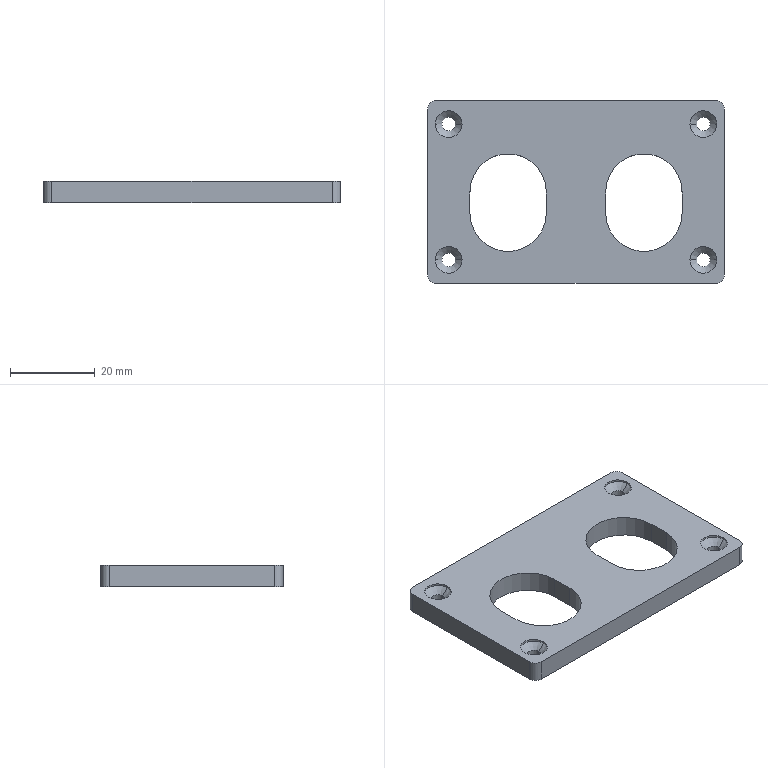Part | SolidWorks | features Extrusion 1, HoleWzd 1 | 1 solid | 42 faces | box 70 x 43 x 5 mm | volume 11317 mm3 | cylinder 24 | plane 10 | cone 8 | commonest cylinder face diameters 3.2 x8 6.3 x8 4 x4 18 x4
STEP:
#1=CARTESIAN_POINT('',(1.85,37.5,4.5));
#2=VERTEX_POINT('',#1);
#3=CARTESIAN_POINT('',(8.15,37.5,4.5));
#4=VERTEX_POINT('',#3);
#5=CARTESIAN_POINT('',(5.,37.5,4.5));
#6=DIRECTION('',(0.,0.,1.));
#7=DIRECTION('',(1.,0.,0.));
#8=AXIS2_PLACEMENT_3D('',#5,#6,#7);
#9=CIRCLE('',#8,3.15);
#10=EDGE_CURVE('',#2,#4,#9,.T.);
#11=ORIENTED_EDGE('',*,*,#10,.F.);
#12=CARTESIAN_POINT('',(1.85,37.5,5.));
#13=VERTEX_POINT('',#12);
#14=CARTESIAN_POINT('',(1.85,37.5,5.));
#15=DIRECTION('',(0.,0.,1.));
#16=VECTOR('',#15,1000.);
#17=LINE('',#14,#16);
#18=EDGE_CURVE('',#2,#13,#17,.T.);
#19=ORIENTED_EDGE('',*,*,#18,.T.);
#20=CARTESIAN_POINT('',(8.15,37.5,5.));
#21=VERTEX_POINT('',#20);
#22=CARTESIAN_POINT('',(5.,37.5,5.));
#23=DIRECTION('',(0.,0.,1.));
#24=DIRECTION('',(1.,0.,0.));
#25=AXIS2_PLACEMENT_3D('',#22,#23,#24);
#26=CIRCLE('',#25,3.15);
#27=EDGE_CURVE('',#13,#21,#26,.T.);
#28=ORIENTED_EDGE('',*,*,#27,.T.);
#29=CARTESIAN_POINT('',(8.15,37.5,5.));
#30=DIRECTION('',(0.,0.,1.));
#31=VECTOR('',#30,1000.);
#32=LINE('',#29,#31);
#33=EDGE_CURVE('',#4,#21,#32,.T.);
#34=ORIENTED_EDGE('',*,*,#33,.F.);
#35=EDGE_LOOP('',(#11,#19,#28,#34));
#36=FACE_OUTER_BOUND('',#35,.T.);
#37=CARTESIAN_POINT('',(5.,37.5,5.));
#38=DIRECTION('',(0.,0.,1.));
#39=DIRECTION('',(1.,0.,0.));
#40=AXIS2_PLACEMENT_3D('',#37,#38,#39);
#41=CYLINDRICAL_SURFACE('',#40,3.15);
#42=ADVANCED_FACE('',(#36),#41,.F.);
#43=CARTESIAN_POINT('',(3.4,37.5,2.95));
#44=VERTEX_POINT('',#43);
#45=CARTESIAN_POINT('',(6.6,37.5,2.95));
#46=VERTEX_POINT('',#45);
#47=CARTESIAN_POINT('',(5.,37.5,2.95));
#48=DIRECTION('',(0.,0.,1.));
#49=DIRECTION('',(1.,0.,0.));
#50=AXIS2_PLACEMENT_3D('',#47,#48,#49);
#51=CIRCLE('',#50,1.6);
#52=EDGE_CURVE('',#44,#46,#51,.T.);
#53=ORIENTED_EDGE('',*,*,#52,.F.);
#54=CARTESIAN_POINT('',(1.85,37.5,4.5));
#55=DIRECTION('',(-0.7071,0.,0.7071));
#56=VECTOR('',#55,1000.);
#57=LINE('',#54,#56);
#58=EDGE_CURVE('',#44,#2,#57,.T.);
#59=ORIENTED_EDGE('',*,*,#58,.T.);
#60=ORIENTED_EDGE('',*,*,#10,.T.);
#61=CARTESIAN_POINT('',(8.15,37.5,4.5));
#62=DIRECTION('',(0.7071,0.,0.7071));
#63=VECTOR('',#62,1000.);
#64=LINE('',#61,#63);
#65=EDGE_CURVE('',#46,#4,#64,.T.);
#66=ORIENTED_EDGE('',*,*,#65,.F.);
#67=EDGE_LOOP('',(#53,#59,#60,#66));
#68=FACE_OUTER_BOUND('',#67,.T.);
#69=CARTESIAN_POINT('',(5.,37.5,4.5));
#70=DIRECTION('',(0.,0.,1.));
#71=DIRECTION('',(1.,0.,0.));
#72=AXIS2_PLACEMENT_3D('',#69,#70,#71);
#73=CONICAL_SURFACE('',#72,3.15,0.7854);
#74=ADVANCED_FACE('',(#68),#73,.F.);
#75=CARTESIAN_POINT('',(3.4,37.5,0.));
#76=VERTEX_POINT('',#75);
#77=CARTESIAN_POINT('',(6.6,37.5,0.));
#78=VERTEX_POINT('',#77);
#79=CARTESIAN_POINT('',(5.,37.5,0.));
#80=DIRECTION('',(0.,0.,1.));
#81=DIRECTION('',(1.,0.,0.));
#82=AXIS2_PLACEMENT_3D('',#79,#80,#81);
#83=CIRCLE('',#82,1.6);
#84=EDGE_CURVE('',#76,#78,#83,.T.);
#85=ORIENTED_EDGE('',*,*,#84,.F.);
#86=CARTESIAN_POINT('',(3.4,37.5,5.));
#87=DIRECTION('',(0.,0.,1.));
#88=VECTOR('',#87,1000.);
#89=LINE('',#86,#88);
#90=EDGE_CURVE('',#76,#44,#89,.T.);
#91=ORIENTED_EDGE('',*,*,#90,.T.);
#92=ORIENTED_EDGE('',*,*,#52,.T.);
#93=CARTESIAN_POINT('',(6.6,37.5,5.));
#94=DIRECTION('',(0.,0.,1.));
#95=VECTOR('',#94,1000.);
#96=LINE('',#93,#95);
#97=EDGE_CURVE('',#78,#46,#96,.T.);
#98=ORIENTED_EDGE('',*,*,#97,.F.);
#99=EDGE_LOOP('',(#85,#91,#92,#98));
#100=FACE_OUTER_BOUND('',#99,.T.);
#101=CARTESIAN_POINT('',(5.,37.5,5.));
#102=DIRECTION('',(0.,0.,1.));
#103=DIRECTION('',(1.,0.,0.));
#104=AXIS2_PLACEMENT_3D('',#101,#102,#103);
#105=CYLINDRICAL_SURFACE('',#104,1.6);
#106=ADVANCED_FACE('',(#100),#105,.F.);
#107=CARTESIAN_POINT('',(1.85,5.5,4.5));
#108=VERTEX_POINT('',#107);
#109=CARTESIAN_POINT('',(8.15,5.5,4.5));
#110=VERTEX_POINT('',#109);
#111=CARTESIAN_POINT('',(5.,5.5,4.5));
#112=DIRECTION('',(0.,0.,1.));
#113=DIRECTION('',(1.,0.,0.));
#114=AXIS2_PLACEMENT_3D('',#111,#112,#113);
#115=CIRCLE('',#114,3.15);
#116=EDGE_CURVE('',#108,#110,#115,.T.);
#117=ORIENTED_EDGE('',*,*,#116,.F.);
#118=CARTESIAN_POINT('',(1.85,5.5,5.));
#119=VERTEX_POINT('',#118);
#120=CARTESIAN_POINT('',(1.85,5.5,5.));
#121=DIRECTION('',(0.,0.,1.));
#122=VECTOR('',#121,1000.);
#123=LINE('',#120,#122);
#124=EDGE_CURVE('',#108,#119,#123,.T.);
#125=ORIENTED_EDGE('',*,*,#124,.T.);
#126=CARTESIAN_POINT('',(8.15,5.5,5.));
#127=VERTEX_POINT('',#126);
#128=CARTESIAN_POINT('',(5.,5.5,5.));
#129=DIRECTION('',(0.,0.,1.));
#130=DIRECTION('',(1.,0.,0.));
#131=AXIS2_PLACEMENT_3D('',#128,#129,#130);
#132=CIRCLE('',#131,3.15);
#133=EDGE_CURVE('',#119,#127,#132,.T.);
#134=ORIENTED_EDGE('',*,*,#133,.T.);
#135=CARTESIAN_POINT('',(8.15,5.5,5.));
#136=DIRECTION('',(0.,0.,1.));
#137=VECTOR('',#136,1000.);
#138=LINE('',#135,#137);
#139=EDGE_CURVE('',#110,#127,#138,.T.);
#140=ORIENTED_EDGE('',*,*,#139,.F.);
#141=EDGE_LOOP('',(#117,#125,#134,#140));
#142=FACE_OUTER_BOUND('',#141,.T.);
#143=CARTESIAN_POINT('',(5.,5.5,5.));
#144=DIRECTION('',(0.,0.,1.));
#145=DIRECTION('',(1.,0.,0.));
#146=AXIS2_PLACEMENT_3D('',#143,#144,#145);
#147=CYLINDRICAL_SURFACE('',#146,3.15);
#148=ADVANCED_FACE('',(#142),#147,.F.);
#149=CARTESIAN_POINT('',(3.4,5.5,2.95));
#150=VERTEX_POINT('',#149);
#151=CARTESIAN_POINT('',(6.6,5.5,2.95));
#152=VERTEX_POINT('',#151);
#153=CARTESIAN_POINT('',(5.,5.5,2.95));
#154=DIRECTION('',(0.,0.,1.));
#155=DIRECTION('',(1.,0.,0.));
#156=AXIS2_PLACEMENT_3D('',#153,#154,#155);
#157=CIRCLE('',#156,1.6);
#158=EDGE_CURVE('',#150,#152,#157,.T.);
#159=ORIENTED_EDGE('',*,*,#158,.F.);
#160=CARTESIAN_POINT('',(1.85,5.5,4.5));
#161=DIRECTION('',(-0.7071,0.,0.7071));
#162=VECTOR('',#161,1000.);
#163=LINE('',#160,#162);
#164=EDGE_CURVE('',#150,#108,#163,.T.);
#165=ORIENTED_EDGE('',*,*,#164,.T.);
#166=ORIENTED_EDGE('',*,*,#116,.T.);
#167=CARTESIAN_POINT('',(8.15,5.5,4.5));
#168=DIRECTION('',(0.7071,0.,0.7071));
#169=VECTOR('',#168,1000.);
#170=LINE('',#167,#169);
#171=EDGE_CURVE('',#152,#110,#170,.T.);
#172=ORIENTED_EDGE('',*,*,#171,.F.);
#173=EDGE_LOOP('',(#159,#165,#166,#172));
#174=FACE_OUTER_BOUND('',#173,.T.);
#175=CARTESIAN_POINT('',(5.,5.5,4.5));
#176=DIRECTION('',(0.,0.,1.));
#177=DIRECTION('',(1.,0.,0.));
#178=AXIS2_PLACEMENT_3D('',#175,#176,#177);
#179=CONICAL_SURFACE('',#178,3.15,0.7854);
#180=ADVANCED_FACE('',(#174),#179,.F.);
#181=CARTESIAN_POINT('',(3.4,5.5,0.));
#182=VERTEX_POINT('',#181);
#183=CARTESIAN_POINT('',(6.6,5.5,0.));
#184=VERTEX_POINT('',#183);
#185=CARTESIAN_POINT('',(5.,5.5,0.));
#186=DIRECTION('',(0.,0.,1.));
#187=DIRECTION('',(1.,0.,0.));
#188=AXIS2_PLACEMENT_3D('',#185,#186,#187);
#189=CIRCLE('',#188,1.6);
#190=EDGE_CURVE('',#182,#184,#189,.T.);
#191=ORIENTED_EDGE('',*,*,#190,.F.);
#192=CARTESIAN_POINT('',(3.4,5.5,5.));
#193=DIRECTION('',(0.,0.,1.));
#194=VECTOR('',#193,1000.);
#195=LINE('',#192,#194);
#196=EDGE_CURVE('',#182,#150,#195,.T.);
#197=ORIENTED_EDGE('',*,*,#196,.T.);
#198=ORIENTED_EDGE('',*,*,#158,.T.);
#199=CARTESIAN_POINT('',(6.6,5.5,5.));
#200=DIRECTION('',(0.,0.,1.));
#201=VECTOR('',#200,1000.);
#202=LINE('',#199,#201);
#203=EDGE_CURVE('',#184,#152,#202,.T.);
#204=ORIENTED_EDGE('',*,*,#203,.F.);
#205=EDGE_LOOP('',(#191,#197,#198,#204));
#206=FACE_OUTER_BOUND('',#205,.T.);
#207=CARTESIAN_POINT('',(5.,5.5,5.));
#208=DIRECTION('',(0.,0.,1.));
#209=DIRECTION('',(1.,0.,0.));
#210=AXIS2_PLACEMENT_3D('',#207,#208,#209);
#211=CYLINDRICAL_SURFACE('',#210,1.6);
#212=ADVANCED_FACE('',(#206),#211,.F.);
#213=CARTESIAN_POINT('',(61.85,5.5,4.5));
#214=VERTEX_POINT('',#213);
#215=CARTESIAN_POINT('',(68.15,5.5,4.5));
#216=VERTEX_POINT('',#215);
#217=CARTESIAN_POINT('',(65.,5.5,4.5));
#218=DIRECTION('',(0.,0.,1.));
#219=DIRECTION('',(1.,0.,0.));
#220=AXIS2_PLACEMENT_3D('',#217,#218,#219);
#221=CIRCLE('',#220,3.15);
#222=EDGE_CURVE('',#214,#216,#221,.T.);
#223=ORIENTED_EDGE('',*,*,#222,.F.);
#224=CARTESIAN_POINT('',(61.85,5.5,5.));
#225=VERTEX_POINT('',#224);
#226=CARTESIAN_POINT('',(61.85,5.5,5.));
#227=DIRECTION('',(0.,0.,1.));
#228=VECTOR('',#227,1000.);
#229=LINE('',#226,#228);
#230=EDGE_CURVE('',#214,#225,#229,.T.);
#231=ORIENTED_EDGE('',*,*,#230,.T.);
#232=CARTESIAN_POINT('',(68.15,5.5,5.));
#233=VERTEX_POINT('',#232);
#234=CARTESIAN_POINT('',(65.,5.5,5.));
#235=DIRECTION('',(0.,0.,1.));
#236=DIRECTION('',(1.,0.,0.));
#237=AXIS2_PLACEMENT_3D('',#234,#235,#236);
#238=CIRCLE('',#237,3.15);
#239=EDGE_CURVE('',#225,#233,#238,.T.);
#240=ORIENTED_EDGE('',*,*,#239,.T.);
#241=CARTESIAN_POINT('',(68.15,5.5,5.));
#242=DIRECTION('',(0.,0.,1.));
#243=VECTOR('',#242,1000.);
#244=LINE('',#241,#243);
#245=EDGE_CURVE('',#216,#233,#244,.T.);
#246=ORIENTED_EDGE('',*,*,#245,.F.);
#247=EDGE_LOOP('',(#223,#231,#240,#246));
#248=FACE_OUTER_BOUND('',#247,.T.);
#249=CARTESIAN_POINT('',(65.,5.5,5.));
#250=DIRECTION('',(0.,0.,1.));
#251=DIRECTION('',(1.,0.,0.));
#252=AXIS2_PLACEMENT_3D('',#249,#250,#251);
#253=CYLINDRICAL_SURFACE('',#252,3.15);
#254=ADVANCED_FACE('',(#248),#253,.F.);
#255=CARTESIAN_POINT('',(63.4,5.5,2.95));
#256=VERTEX_POINT('',#255);
#257=CARTESIAN_POINT('',(66.6,5.5,2.95));
#258=VERTEX_POINT('',#257);
#259=CARTESIAN_POINT('',(65.,5.5,2.95));
#260=DIRECTION('',(0.,0.,1.));
#261=DIRECTION('',(1.,0.,0.));
#262=AXIS2_PLACEMENT_3D('',#259,#260,#261);
#263=CIRCLE('',#262,1.6);
#264=EDGE_CURVE('',#256,#258,#263,.T.);
#265=ORIENTED_EDGE('',*,*,#264,.F.);
#266=CARTESIAN_POINT('',(61.85,5.5,4.5));
#267=DIRECTION('',(-0.7071,0.,0.7071));
#268=VECTOR('',#267,1000.);
#269=LINE('',#266,#268);
#270=EDGE_CURVE('',#256,#214,#269,.T.);
#271=ORIENTED_EDGE('',*,*,#270,.T.);
#272=ORIENTED_EDGE('',*,*,#222,.T.);
#273=CARTESIAN_POINT('',(68.15,5.5,4.5));
#274=DIRECTION('',(0.7071,0.,0.7071));
#275=VECTOR('',#274,1000.);
#276=LINE('',#273,#275);
#277=EDGE_CURVE('',#258,#216,#276,.T.);
#278=ORIENTED_EDGE('',*,*,#277,.F.);
#279=EDGE_LOOP('',(#265,#271,#272,#278));
#280=FACE_OUTER_BOUND('',#279,.T.);
#281=CARTESIAN_POINT('',(65.,5.5,4.5));
#282=DIRECTION('',(0.,0.,1.));
#283=DIRECTION('',(1.,0.,0.));
#284=AXIS2_PLACEMENT_3D('',#281,#282,#283);
#285=CONICAL_SURFACE('',#284,3.15,0.7854);
#286=ADVANCED_FACE('',(#280),#285,.F.);
#287=CARTESIAN_POINT('',(63.4,5.5,0.));
#288=VERTEX_POINT('',#287);
#289=CARTESIAN_POINT('',(66.6,5.5,0.));
#290=VERTEX_POINT('',#289);
#291=CARTESIAN_POINT('',(65.,5.5,0.));
#292=DIRECTION('',(0.,0.,1.));
#293=DIRECTION('',(1.,0.,0.));
#294=AXIS2_PLACEMENT_3D('',#291,#292,#293);
#295=CIRCLE('',#294,1.6);
#296=EDGE_CURVE('',#288,#290,#295,.T.);
#297=ORIENTED_EDGE('',*,*,#296,.F.);
#298=CARTESIAN_POINT('',(63.4,5.5,5.));
#299=DIRECTION('',(0.,0.,1.));
#300=VECTOR('',#299,1000.);
#301=LINE('',#298,#300);
#302=EDGE_CURVE('',#288,#256,#301,.T.);
#303=ORIENTED_EDGE('',*,*,#302,.T.);
#304=ORIENTED_EDGE('',*,*,#264,.T.);
#305=CARTESIAN_POINT('',(66.6,5.5,5.));
#306=DIRECTION('',(0.,0.,1.));
#307=VECTOR('',#306,1000.);
#308=LINE('',#305,#307);
#309=EDGE_CURVE('',#290,#258,#308,.T.);
#310=ORIENTED_EDGE('',*,*,#309,.F.);
#311=EDGE_LOOP('',(#297,#303,#304,#310));
#312=FACE_OUTER_BOUND('',#311,.T.);
#313=CARTESIAN_POINT('',(65.,5.5,5.));
#314=DIRECTION('',(0.,0.,1.));
#315=DIRECTION('',(1.,0.,0.));
#316=AXIS2_PLACEMENT_3D('',#313,#314,#315);
#317=CYLINDRICAL_SURFACE('',#316,1.6);
#318=ADVANCED_FACE('',(#312),#317,.F.);
#319=CARTESIAN_POINT('',(61.85,37.5,4.5));
#320=VERTEX_POINT('',#319);
#321=CARTESIAN_POINT('',(68.15,37.5,4.5));
#322=VERTEX_POINT('',#321);
#323=CARTESIAN_POINT('',(65.,37.5,4.5));
#324=DIRECTION('',(0.,0.,1.));
#325=DIRECTION('',(1.,0.,0.));
#326=AXIS2_PLACEMENT_3D('',#323,#324,#325);
#327=CIRCLE('',#326,3.15);
#328=EDGE_CURVE('',#320,#322,#327,.T.);
#329=ORIENTED_EDGE('',*,*,#328,.F.);
#330=CARTESIAN_POINT('',(61.85,37.5,5.));
#331=VERTEX_POINT('',#330);
#332=CARTESIAN_POINT('',(61.85,37.5,5.));
#333=DIRECTION('',(0.,0.,1.));
#334=VECTOR('',#333,1000.);
#335=LINE('',#332,#334);
#336=EDGE_CURVE('',#320,#331,#335,.T.);
#337=ORIENTED_EDGE('',*,*,#336,.T.);
#338=CARTESIAN_POINT('',(68.15,37.5,5.));
#339=VERTEX_POINT('',#338);
#340=CARTESIAN_POINT('',(65.,37.5,5.));
#341=DIRECTION('',(0.,0.,1.));
#342=DIRECTION('',(1.,0.,0.));
#343=AXIS2_PLACEMENT_3D('',#340,#341,#342);
#344=CIRCLE('',#343,3.15);
#345=EDGE_CURVE('',#331,#339,#344,.T.);
#346=ORIENTED_EDGE('',*,*,#345,.T.);
#347=CARTESIAN_POINT('',(68.15,37.5,5.));
#348=DIRECTION('',(0.,0.,1.));
#349=VECTOR('',#348,1000.);
#350=LINE('',#347,#349);
#351=EDGE_CURVE('',#322,#339,#350,.T.);
#352=ORIENTED_EDGE('',*,*,#351,.F.);
#353=EDGE_LOOP('',(#329,#337,#346,#352));
#354=FACE_OUTER_BOUND('',#353,.T.);
#355=CARTESIAN_POINT('',(65.,37.5,5.));
#356=DIRECTION('',(0.,0.,1.));
#357=DIRECTION('',(1.,0.,0.));
#358=AXIS2_PLACEMENT_3D('',#355,#356,#357);
#359=CYLINDRICAL_SURFACE('',#358,3.15);
#360=ADVANCED_FACE('',(#354),#359,.F.);
#361=CARTESIAN_POINT('',(63.4,37.5,2.95));
#362=VERTEX_POINT('',#361);
#363=CARTESIAN_POINT('',(66.6,37.5,2.95));
#364=VERTEX_POINT('',#363);
#365=CARTESIAN_POINT('',(65.,37.5,2.95));
#366=DIRECTION('',(0.,0.,1.));
#367=DIRECTION('',(1.,0.,0.));
#368=AXIS2_PLACEMENT_3D('',#365,#366,#367);
#369=CIRCLE('',#368,1.6);
#370=EDGE_CURVE('',#362,#364,#369,.T.);
#371=ORIENTED_EDGE('',*,*,#370,.F.);
#372=CARTESIAN_POINT('',(61.85,37.5,4.5));
#373=DIRECTION('',(-0.7071,0.,0.7071));
#374=VECTOR('',#373,1000.);
#375=LINE('',#372,#374);
#376=EDGE_CURVE('',#362,#320,#375,.T.);
#377=ORIENTED_EDGE('',*,*,#376,.T.);
#378=ORIENTED_EDGE('',*,*,#328,.T.);
#379=CARTESIAN_POINT('',(68.15,37.5,4.5));
#380=DIRECTION('',(0.7071,0.,0.7071));
#381=VECTOR('',#380,1000.);
#382=LINE('',#379,#381);
#383=EDGE_CURVE('',#364,#322,#382,.T.);
#384=ORIENTED_EDGE('',*,*,#383,.F.);
#385=EDGE_LOOP('',(#371,#377,#378,#384));
#386=FACE_OUTER_BOUND('',#385,.T.);
#387=CARTESIAN_POINT('',(65.,37.5,4.5));
#388=DIRECTION('',(0.,0.,1.));
#389=DIRECTION('',(1.,0.,0.));
#390=AXIS2_PLACEMENT_3D('',#387,#388,#389);
#391=CONICAL_SURFACE('',#390,3.15,0.7854);
#392=ADVANCED_FACE('',(#386),#391,.F.);
#393=CARTESIAN_POINT('',(63.4,37.5,0.));
#394=VERTEX_POINT('',#393);
#395=CARTESIAN_POINT('',(66.6,37.5,0.));
#396=VERTEX_POINT('',#395);
#397=CARTESIAN_POINT('',(65.,37.5,0.));
#398=DIRECTION('',(0.,0.,1.));
#399=DIRECTION('',(1.,0.,0.));
#400=AXIS2_PLACEMENT_3D('',#397,#398,#399);
#401=CIRCLE('',#400,1.6);
#402=EDGE_CURVE('',#394,#396,#401,.T.);
#403=ORIENTED_EDGE('',*,*,#402,.F.);
#404=CARTESIAN_POINT('',(63.4,37.5,5.));
#405=DIRECTION('',(0.,0.,1.));
#406=VECTOR('',#405,1000.);
#407=LINE('',#404,#406);
#408=EDGE_CURVE('',#394,#362,#407,.T.);
#409=ORIENTED_EDGE('',*,*,#408,.T.);
#410=ORIENTED_EDGE('',*,*,#370,.T.);
#411=CARTESIAN_POINT('',(66.6,37.5,5.));
#412=DIRECTION('',(0.,0.,1.));
#413=VECTOR('',#412,1000.);
#414=LINE('',#411,#413);
#415=EDGE_CURVE('',#396,#364,#414,.T.);
#416=ORIENTED_EDGE('',*,*,#415,.F.);
#417=EDGE_LOOP('',(#403,#409,#410,#416));
#418=FACE_OUTER_BOUND('',#417,.T.);
#419=CARTESIAN_POINT('',(65.,37.5,5.));
#420=DIRECTION('',(0.,0.,1.));
#421=DIRECTION('',(1.,0.,0.));
#422=AXIS2_PLACEMENT_3D('',#419,#420,#421);
#423=CYLINDRICAL_SURFACE('',#422,1.6);
#424=ADVANCED_FACE('',(#418),#423,.F.);
#425=CARTESIAN_POINT('',(5.,37.5,5.));
#426=DIRECTION('',(0.,0.,1.));
#427=DIRECTION('',(1.,0.,0.));
#428=AXIS2_PLACEMENT_3D('',#425,#426,#427);
#429=CIRCLE('',#428,3.15);
#430=EDGE_CURVE('',#21,#13,#429,.T.);
#431=ORIENTED_EDGE('',*,*,#430,.F.);
#432=ORIENTED_EDGE('',*,*,#27,.F.);
#433=EDGE_LOOP('',(#431,#432));
#434=FACE_BOUND('',#433,.T.);
#435=CARTESIAN_POINT('',(5.,5.5,5.));
#436=DIRECTION('',(0.,0.,1.));
#437=DIRECTION('',(1.,0.,0.));
#438=AXIS2_PLACEMENT_3D('',#435,#436,#437);
#439=CIRCLE('',#438,3.15);
#440=EDGE_CURVE('',#127,#119,#439,.T.);
#441=ORIENTED_EDGE('',*,*,#440,.F.);
#442=ORIENTED_EDGE('',*,*,#133,.F.);
#443=EDGE_LOOP('',(#441,#442));
#444=FACE_BOUND('',#443,.T.);
#445=CARTESIAN_POINT('',(65.,5.5,5.));
#446=DIRECTION('',(0.,0.,1.));
#447=DIRECTION('',(1.,0.,0.));
#448=AXIS2_PLACEMENT_3D('',#445,#446,#447);
#449=CIRCLE('',#448,3.15);
#450=EDGE_CURVE('',#233,#225,#449,.T.);
#451=ORIENTED_EDGE('',*,*,#450,.F.);
#452=ORIENTED_EDGE('',*,*,#239,.F.);
#453=EDGE_LOOP('',(#451,#452));
#454=FACE_BOUND('',#453,.T.);
#455=CARTESIAN_POINT('',(65.,37.5,5.));
#456=DIRECTION('',(0.,0.,1.));
#457=DIRECTION('',(1.,0.,0.));
#458=AXIS2_PLACEMENT_3D('',#455,#456,#457);
#459=CIRCLE('',#458,3.15);
#460=EDGE_CURVE('',#339,#331,#459,.T.);
#461=ORIENTED_EDGE('',*,*,#460,.F.);
#462=ORIENTED_EDGE('',*,*,#345,.F.);
#463=EDGE_LOOP('',(#461,#462));
#464=FACE_BOUND('',#463,.T.);
#465=CARTESIAN_POINT('',(28.,21.5,5.));
#466=VERTEX_POINT('',#465);
#467=CARTESIAN_POINT('',(10.,21.5,5.));
#468=VERTEX_POINT('',#467);
#469=CARTESIAN_POINT('',(19.,21.5,5.));
#470=DIRECTION('',(0.,0.,1.));
#471=DIRECTION('',(1.,0.,0.));
#472=AXIS2_PLACEMENT_3D('',#469,#470,#471);
#473=CIRCLE('',#472,9.);
#474=EDGE_CURVE('',#466,#468,#473,.T.);
#475=ORIENTED_EDGE('',*,*,#474,.F.);
#476=CARTESIAN_POINT('',(28.,16.5,5.));
#477=VERTEX_POINT('',#476);
#478=CARTESIAN_POINT('',(28.,21.5,5.));
#479=DIRECTION('',(0.,1.,0.));
#480=VECTOR('',#479,1000.);
#481=LINE('',#478,#480);
#482=EDGE_CURVE('',#477,#466,#481,.T.);
#483=ORIENTED_EDGE('',*,*,#482,.F.);
#484=CARTESIAN_POINT('',(10.,16.5,5.));
#485=VERTEX_POINT('',#484);
#486=CARTESIAN_POINT('',(19.,16.5,5.));
#487=DIRECTION('',(0.,0.,1.));
#488=DIRECTION('',(1.,0.,0.));
#489=AXIS2_PLACEMENT_3D('',#486,#487,#488);
#490=CIRCLE('',#489,9.);
#491=EDGE_CURVE('',#485,#477,#490,.T.);
#492=ORIENTED_EDGE('',*,*,#491,.F.);
#493=CARTESIAN_POINT('',(10.,21.5,5.));
#494=DIRECTION('',(0.,-1.,0.));
#495=VECTOR('',#494,1000.);
#496=LINE('',#493,#495);
#497=EDGE_CURVE('',#468,#485,#496,.T.);
#498=ORIENTED_EDGE('',*,*,#497,.F.);
#499=EDGE_LOOP('',(#475,#483,#492,#498));
#500=FACE_BOUND('',#499,.T.);
#501=CARTESIAN_POINT('',(70.,41.,5.));
#502=VERTEX_POINT('',#501);
#503=CARTESIAN_POINT('',(68.,43.,5.));
#504=VERTEX_POINT('',#503);
#505=CARTESIAN_POINT('',(68.,41.,5.));
#506=DIRECTION('',(0.,0.,1.));
#507=DIRECTION('',(-1.,0.,0.));
#508=AXIS2_PLACEMENT_3D('',#505,#506,#507);
#509=CIRCLE('',#508,2.);
#510=EDGE_CURVE('',#502,#504,#509,.T.);
#511=ORIENTED_EDGE('',*,*,#510,.T.);
#512=CARTESIAN_POINT('',(2.,43.,5.));
#513=VERTEX_POINT('',#512);
#514=CARTESIAN_POINT('',(2.,43.,5.));
#515=DIRECTION('',(-1.,0.,0.));
#516=VECTOR('',#515,1000.);
#517=LINE('',#514,#516);
#518=EDGE_CURVE('',#504,#513,#517,.T.);
#519=ORIENTED_EDGE('',*,*,#518,.T.);
#520=CARTESIAN_POINT('',(0.,41.,5.));
#521=VERTEX_POINT('',#520);
#522=CARTESIAN_POINT('',(2.,41.,5.));
#523=DIRECTION('',(0.,0.,1.));
#524=DIRECTION('',(-1.,0.,0.));
#525=AXIS2_PLACEMENT_3D('',#522,#523,#524);
#526=CIRCLE('',#525,2.);
#527=EDGE_CURVE('',#513,#521,#526,.T.);
#528=ORIENTED_EDGE('',*,*,#527,.T.);
#529=CARTESIAN_POINT('',(0.,2.,5.));
#530=VERTEX_POINT('',#529);
#531=CARTESIAN_POINT('',(0.,2.,5.));
#532=DIRECTION('',(0.,-1.,0.));
#533=VECTOR('',#532,1000.);
#534=LINE('',#531,#533);
#535=EDGE_CURVE('',#521,#530,#534,.T.);
#536=ORIENTED_EDGE('',*,*,#535,.T.);
#537=CARTESIAN_POINT('',(2.,0.,5.));
#538=VERTEX_POINT('',#537);
#539=CARTESIAN_POINT('',(2.,2.,5.));
#540=DIRECTION('',(0.,0.,1.));
#541=DIRECTION('',(-1.,0.,0.));
#542=AXIS2_PLACEMENT_3D('',#539,#540,#541);
#543=CIRCLE('',#542,2.);
#544=EDGE_CURVE('',#530,#538,#543,.T.);
#545=ORIENTED_EDGE('',*,*,#544,.T.);
#546=CARTESIAN_POINT('',(68.,0.,5.));
#547=VERTEX_POINT('',#546);
#548=CARTESIAN_POINT('',(2.,0.,5.));
#549=DIRECTION('',(1.,0.,0.));
#550=VECTOR('',#549,1000.);
#551=LINE('',#548,#550);
#552=EDGE_CURVE('',#538,#547,#551,.T.);
#553=ORIENTED_EDGE('',*,*,#552,.T.);
#554=CARTESIAN_POINT('',(70.,2.,5.));
#555=VERTEX_POINT('',#554);
#556=CARTESIAN_POINT('',(68.,2.,5.));
#557=DIRECTION('',(0.,0.,1.));
#558=DIRECTION('',(1.,0.,0.));
#559=AXIS2_PLACEMENT_3D('',#556,#557,#558);
#560=CIRCLE('',#559,2.);
#561=EDGE_CURVE('',#547,#555,#560,.T.);
#562=ORIENTED_EDGE('',*,*,#561,.T.);
#563=CARTESIAN_POINT('',(70.,2.,5.));
#564=DIRECTION('',(0.,1.,0.));
#565=VECTOR('',#564,1000.);
#566=LINE('',#563,#565);
#567=EDGE_CURVE('',#555,#502,#566,.T.);
#568=ORIENTED_EDGE('',*,*,#567,.T.);
#569=EDGE_LOOP('',(#511,#519,#528,#536,#545,#553,#562,#568));
#570=FACE_OUTER_BOUND('',#569,.T.);
#571=CARTESIAN_POINT('',(60.,21.5,5.));
#572=VERTEX_POINT('',#571);
#573=CARTESIAN_POINT('',(42.,21.5,5.));
#574=VERTEX_POINT('',#573);
#575=CARTESIAN_POINT('',(51.,21.5,5.));
#576=DIRECTION('',(0.,0.,1.));
#577=DIRECTION('',(1.,0.,0.));
#578=AXIS2_PLACEMENT_3D('',#575,#576,#577);
#579=CIRCLE('',#578,9.);
#580=EDGE_CURVE('',#572,#574,#579,.T.);
#581=ORIENTED_EDGE('',*,*,#580,.F.);
#582=CARTESIAN_POINT('',(60.,16.5,5.));
#583=VERTEX_POINT('',#582);
#584=CARTESIAN_POINT('',(60.,21.5,5.));
#585=DIRECTION('',(0.,1.,0.));
#586=VECTOR('',#585,1000.);
#587=LINE('',#584,#586);
#588=EDGE_CURVE('',#583,#572,#587,.T.);
#589=ORIENTED_EDGE('',*,*,#588,.F.);
#590=CARTESIAN_POINT('',(42.,16.5,5.));
#591=VERTEX_POINT('',#590);
#592=CARTESIAN_POINT('',(51.,16.5,5.));
#593=DIRECTION('',(0.,0.,1.));
#594=DIRECTION('',(1.,0.,0.));
#595=AXIS2_PLACEMENT_3D('',#592,#593,#594);
#596=CIRCLE('',#595,9.);
#597=EDGE_CURVE('',#591,#583,#596,.T.);
#598=ORIENTED_EDGE('',*,*,#597,.F.);
#599=CARTESIAN_POINT('',(42.,21.5,5.));
#600=DIRECTION('',(0.,-1.,0.));
#601=VECTOR('',#600,1000.);
#602=LINE('',#599,#601);
#603=EDGE_CURVE('',#574,#591,#602,.T.);
#604=ORIENTED_EDGE('',*,*,#603,.F.);
#605=EDGE_LOOP('',(#581,#589,#598,#604));
#606=FACE_BOUND('',#605,.T.);
#607=CARTESIAN_POINT('',(68.,41.,5.));
#608=DIRECTION('',(0.,0.,-1.));
#609=DIRECTION('',(-1.,0.,0.));
#610=AXIS2_PLACEMENT_3D('',#607,#608,#609);
#611=PLANE('',#610);
#612=ADVANCED_FACE('',(#434,#444,#454,#464,#500,#570,#606),#611,.F.);
#613=CARTESIAN_POINT('',(5.,37.5,0.));
#614=DIRECTION('',(0.,0.,1.));
#615=DIRECTION('',(1.,0.,0.));
#616=AXIS2_PLACEMENT_3D('',#613,#614,#615);
#617=CIRCLE('',#616,1.6);
#618=EDGE_CURVE('',#78,#76,#617,.T.);
#619=ORIENTED_EDGE('',*,*,#618,.T.);
#620=ORIENTED_EDGE('',*,*,#84,.T.);
#621=EDGE_LOOP('',(#619,#620));
#622=FACE_BOUND('',#621,.T.);
#623=CARTESIAN_POINT('',(5.,5.5,0.));
#624=DIRECTION('',(0.,0.,1.));
#625=DIRECTION('',(1.,0.,0.));
#626=AXIS2_PLACEMENT_3D('',#623,#624,#625);
#627=CIRCLE('',#626,1.6);
#628=EDGE_CURVE('',#184,#182,#627,.T.);
#629=ORIENTED_EDGE('',*,*,#628,.T.);
#630=ORIENTED_EDGE('',*,*,#190,.T.);
#631=EDGE_LOOP('',(#629,#630));
#632=FACE_BOUND('',#631,.T.);
#633=CARTESIAN_POINT('',(65.,5.5,0.));
#634=DIRECTION('',(0.,0.,1.));
#635=DIRECTION('',(1.,0.,0.));
#636=AXIS2_PLACEMENT_3D('',#633,#634,#635);
#637=CIRCLE('',#636,1.6);
#638=EDGE_CURVE('',#290,#288,#637,.T.);
#639=ORIENTED_EDGE('',*,*,#638,.T.);
#640=ORIENTED_EDGE('',*,*,#296,.T.);
#641=EDGE_LOOP('',(#639,#640));
#642=FACE_BOUND('',#641,.T.);
#643=CARTESIAN_POINT('',(65.,37.5,0.));
#644=DIRECTION('',(0.,0.,1.));
#645=DIRECTION('',(1.,0.,0.));
#646=AXIS2_PLACEMENT_3D('',#643,#644,#645);
#647=CIRCLE('',#646,1.6);
#648=EDGE_CURVE('',#396,#394,#647,.T.);
#649=ORIENTED_EDGE('',*,*,#648,.T.);
#650=ORIENTED_EDGE('',*,*,#402,.T.);
#651=EDGE_LOOP('',(#649,#650));
#652=FACE_BOUND('',#651,.T.);
#653=CARTESIAN_POINT('',(28.,16.5,0.));
#654=VERTEX_POINT('',#653);
#655=CARTESIAN_POINT('',(28.,21.5,0.));
#656=VERTEX_POINT('',#655);
#657=CARTESIAN_POINT('',(28.,21.5,0.));
#658=DIRECTION('',(0.,1.,0.));
#659=VECTOR('',#658,1000.);
#660=LINE('',#657,#659);
#661=EDGE_CURVE('',#654,#656,#660,.T.);
#662=ORIENTED_EDGE('',*,*,#661,.T.);
#663=CARTESIAN_POINT('',(10.,21.5,0.));
#664=VERTEX_POINT('',#663);
#665=CARTESIAN_POINT('',(19.,21.5,0.));
#666=DIRECTION('',(0.,0.,1.));
#667=DIRECTION('',(1.,0.,0.));
#668=AXIS2_PLACEMENT_3D('',#665,#666,#667);
#669=CIRCLE('',#668,9.);
#670=EDGE_CURVE('',#656,#664,#669,.T.);
#671=ORIENTED_EDGE('',*,*,#670,.T.);
#672=CARTESIAN_POINT('',(10.,16.5,0.));
#673=VERTEX_POINT('',#672);
#674=CARTESIAN_POINT('',(10.,21.5,0.));
#675=DIRECTION('',(0.,-1.,0.));
#676=VECTOR('',#675,1000.);
#677=LINE('',#674,#676);
#678=EDGE_CURVE('',#664,#673,#677,.T.);
#679=ORIENTED_EDGE('',*,*,#678,.T.);
#680=CARTESIAN_POINT('',(19.,16.5,0.));
#681=DIRECTION('',(0.,0.,1.));
#682=DIRECTION('',(1.,0.,0.));
#683=AXIS2_PLACEMENT_3D('',#680,#681,#682);
#684=CIRCLE('',#683,9.);
#685=EDGE_CURVE('',#673,#654,#684,.T.);
#686=ORIENTED_EDGE('',*,*,#685,.T.);
#687=EDGE_LOOP('',(#662,#671,#679,#686));
#688=FACE_BOUND('',#687,.T.);
#689=CARTESIAN_POINT('',(70.,41.,0.));
#690=VERTEX_POINT('',#689);
#691=CARTESIAN_POINT('',(68.,43.,0.));
#692=VERTEX_POINT('',#691);
#693=CARTESIAN_POINT('',(68.,41.,0.));
#694=DIRECTION('',(0.,0.,1.));
#695=DIRECTION('',(-1.,0.,0.));
#696=AXIS2_PLACEMENT_3D('',#693,#694,#695);
#697=CIRCLE('',#696,2.);
#698=EDGE_CURVE('',#690,#692,#697,.T.);
#699=ORIENTED_EDGE('',*,*,#698,.F.);
#700=CARTESIAN_POINT('',(70.,2.,0.));
#701=VERTEX_POINT('',#700);
#702=CARTESIAN_POINT('',(70.,2.,0.));
#703=DIRECTION('',(0.,1.,0.));
#704=VECTOR('',#703,1000.);
#705=LINE('',#702,#704);
#706=EDGE_CURVE('',#701,#690,#705,.T.);
#707=ORIENTED_EDGE('',*,*,#706,.F.);
#708=CARTESIAN_POINT('',(68.,0.,0.));
#709=VERTEX_POINT('',#708);
#710=CARTESIAN_POINT('',(68.,2.,0.));
#711=DIRECTION('',(0.,0.,1.));
#712=DIRECTION('',(1.,0.,0.));
#713=AXIS2_PLACEMENT_3D('',#710,#711,#712);
#714=CIRCLE('',#713,2.);
#715=EDGE_CURVE('',#709,#701,#714,.T.);
#716=ORIENTED_EDGE('',*,*,#715,.F.);
#717=CARTESIAN_POINT('',(2.,0.,0.));
#718=VERTEX_POINT('',#717);
#719=CARTESIAN_POINT('',(2.,0.,0.));
#720=DIRECTION('',(1.,0.,0.));
#721=VECTOR('',#720,1000.);
#722=LINE('',#719,#721);
#723=EDGE_CURVE('',#718,#709,#722,.T.);
#724=ORIENTED_EDGE('',*,*,#723,.F.);
#725=CARTESIAN_POINT('',(0.,2.,0.));
#726=VERTEX_POINT('',#725);
#727=CARTESIAN_POINT('',(2.,2.,0.));
#728=DIRECTION('',(0.,0.,1.));
#729=DIRECTION('',(-1.,0.,0.));
#730=AXIS2_PLACEMENT_3D('',#727,#728,#729);
#731=CIRCLE('',#730,2.);
#732=EDGE_CURVE('',#726,#718,#731,.T.);
#733=ORIENTED_EDGE('',*,*,#732,.F.);
#734=CARTESIAN_POINT('',(0.,41.,0.));
#735=VERTEX_POINT('',#734);
#736=CARTESIAN_POINT('',(0.,2.,0.));
#737=DIRECTION('',(0.,-1.,0.));
#738=VECTOR('',#737,1000.);
#739=LINE('',#736,#738);
#740=EDGE_CURVE('',#735,#726,#739,.T.);
#741=ORIENTED_EDGE('',*,*,#740,.F.);
#742=CARTESIAN_POINT('',(2.,43.,0.));
#743=VERTEX_POINT('',#742);
#744=CARTESIAN_POINT('',(2.,41.,0.));
#745=DIRECTION('',(0.,0.,1.));
#746=DIRECTION('',(-1.,0.,0.));
#747=AXIS2_PLACEMENT_3D('',#744,#745,#746);
#748=CIRCLE('',#747,2.);
#749=EDGE_CURVE('',#743,#735,#748,.T.);
#750=ORIENTED_EDGE('',*,*,#749,.F.);
#751=CARTESIAN_POINT('',(2.,43.,0.));
#752=DIRECTION('',(-1.,0.,0.));
#753=VECTOR('',#752,1000.);
#754=LINE('',#751,#753);
#755=EDGE_CURVE('',#692,#743,#754,.T.);
#756=ORIENTED_EDGE('',*,*,#755,.F.);
#757=EDGE_LOOP('',(#699,#707,#716,#724,#733,#741,#750,#756));
#758=FACE_OUTER_BOUND('',#757,.T.);
#759=CARTESIAN_POINT('',(60.,16.5,0.));
#760=VERTEX_POINT('',#759);
#761=CARTESIAN_POINT('',(60.,21.5,0.));
#762=VERTEX_POINT('',#761);
#763=CARTESIAN_POINT('',(60.,21.5,0.));
#764=DIRECTION('',(0.,1.,0.));
#765=VECTOR('',#764,1000.);
#766=LINE('',#763,#765);
#767=EDGE_CURVE('',#760,#762,#766,.T.);
#768=ORIENTED_EDGE('',*,*,#767,.T.);
#769=CARTESIAN_POINT('',(42.,21.5,0.));
#770=VERTEX_POINT('',#769);
#771=CARTESIAN_POINT('',(51.,21.5,0.));
#772=DIRECTION('',(0.,0.,1.));
#773=DIRECTION('',(1.,0.,0.));
#774=AXIS2_PLACEMENT_3D('',#771,#772,#773);
#775=CIRCLE('',#774,9.);
#776=EDGE_CURVE('',#762,#770,#775,.T.);
#777=ORIENTED_EDGE('',*,*,#776,.T.);
#778=CARTESIAN_POINT('',(42.,16.5,0.));
#779=VERTEX_POINT('',#778);
#780=CARTESIAN_POINT('',(42.,21.5,0.));
#781=DIRECTION('',(0.,-1.,0.));
#782=VECTOR('',#781,1000.);
#783=LINE('',#780,#782);
#784=EDGE_CURVE('',#770,#779,#783,.T.);
#785=ORIENTED_EDGE('',*,*,#784,.T.);
#786=CARTESIAN_POINT('',(51.,16.5,0.));
#787=DIRECTION('',(0.,0.,1.));
#788=DIRECTION('',(1.,0.,0.));
#789=AXIS2_PLACEMENT_3D('',#786,#787,#788);
#790=CIRCLE('',#789,9.);
#791=EDGE_CURVE('',#779,#760,#790,.T.);
#792=ORIENTED_EDGE('',*,*,#791,.T.);
#793=EDGE_LOOP('',(#768,#777,#785,#792));
#794=FACE_BOUND('',#793,.T.);
#795=CARTESIAN_POINT('',(68.,41.,0.));
#796=DIRECTION('',(0.,0.,-1.));
#797=DIRECTION('',(-1.,0.,0.));
#798=AXIS2_PLACEMENT_3D('',#795,#796,#797);
#799=PLANE('',#798);
#800=ADVANCED_FACE('',(#622,#632,#642,#652,#688,#758,#794),#799,.T.);
#801=ORIENTED_EDGE('',*,*,#698,.T.);
#802=CARTESIAN_POINT('',(68.,43.,5.));
#803=DIRECTION('',(0.,0.,-1.));
#804=VECTOR('',#803,1000.);
#805=LINE('',#802,#804);
#806=EDGE_CURVE('',#504,#692,#805,.T.);
#807=ORIENTED_EDGE('',*,*,#806,.F.);
#808=ORIENTED_EDGE('',*,*,#510,.F.);
#809=CARTESIAN_POINT('',(70.,41.,5.));
#810=DIRECTION('',(0.,0.,-1.));
#811=VECTOR('',#810,1000.);
#812=LINE('',#809,#811);
#813=EDGE_CURVE('',#502,#690,#812,.T.);
#814=ORIENTED_EDGE('',*,*,#813,.T.);
#815=EDGE_LOOP('',(#801,#807,#808,#814));
#816=FACE_OUTER_BOUND('',#815,.T.);
#817=CARTESIAN_POINT('',(68.,41.,5.));
#818=DIRECTION('',(0.,0.,-1.));
#819=DIRECTION('',(-1.,0.,0.));
#820=AXIS2_PLACEMENT_3D('',#817,#818,#819);
#821=CYLINDRICAL_SURFACE('',#820,2.);
#822=ADVANCED_FACE('',(#816),#821,.T.);
#823=ORIENTED_EDGE('',*,*,#755,.T.);
#824=CARTESIAN_POINT('',(2.,43.,5.));
#825=DIRECTION('',(0.,0.,-1.));
#826=VECTOR('',#825,1000.);
#827=LINE('',#824,#826);
#828=EDGE_CURVE('',#513,#743,#827,.T.);
#829=ORIENTED_EDGE('',*,*,#828,.F.);
#830=ORIENTED_EDGE('',*,*,#518,.F.);
#831=ORIENTED_EDGE('',*,*,#806,.T.);
#832=EDGE_LOOP('',(#823,#829,#830,#831));
#833=FACE_OUTER_BOUND('',#832,.T.);
#834=CARTESIAN_POINT('',(2.,43.,5.));
#835=DIRECTION('',(0.,-1.,0.));
#836=DIRECTION('',(1.,0.,0.));
#837=AXIS2_PLACEMENT_3D('',#834,#835,#836);
#838=PLANE('',#837);
#839=ADVANCED_FACE('',(#833),#838,.F.);
#840=ORIENTED_EDGE('',*,*,#749,.T.);
#841=CARTESIAN_POINT('',(0.,41.,5.));
#842=DIRECTION('',(0.,0.,-1.));
#843=VECTOR('',#842,1000.);
#844=LINE('',#841,#843);
#845=EDGE_CURVE('',#521,#735,#844,.T.);
#846=ORIENTED_EDGE('',*,*,#845,.F.);
#847=ORIENTED_EDGE('',*,*,#527,.F.);
#848=ORIENTED_EDGE('',*,*,#828,.T.);
#849=EDGE_LOOP('',(#840,#846,#847,#848));
#850=FACE_OUTER_BOUND('',#849,.T.);
#851=CARTESIAN_POINT('',(2.,41.,5.));
#852=DIRECTION('',(0.,0.,-1.));
#853=DIRECTION('',(-1.,0.,0.));
#854=AXIS2_PLACEMENT_3D('',#851,#852,#853);
#855=CYLINDRICAL_SURFACE('',#854,2.);
#856=ADVANCED_FACE('',(#850),#855,.T.);
#857=ORIENTED_EDGE('',*,*,#740,.T.);
#858=CARTESIAN_POINT('',(0.,2.,5.));
#859=DIRECTION('',(0.,0.,-1.));
#860=VECTOR('',#859,1000.);
#861=LINE('',#858,#860);
#862=EDGE_CURVE('',#530,#726,#861,.T.);
#863=ORIENTED_EDGE('',*,*,#862,.F.);
#864=ORIENTED_EDGE('',*,*,#535,.F.);
#865=ORIENTED_EDGE('',*,*,#845,.T.);
#866=EDGE_LOOP('',(#857,#863,#864,#865));
#867=FACE_OUTER_BOUND('',#866,.T.);
#868=CARTESIAN_POINT('',(0.,2.,5.));
#869=DIRECTION('',(1.,0.,0.));
#870=DIRECTION('',(0.,0.,-1.));
#871=AXIS2_PLACEMENT_3D('',#868,#869,#870);
#872=PLANE('',#871);
#873=ADVANCED_FACE('',(#867),#872,.F.);
#874=ORIENTED_EDGE('',*,*,#732,.T.);
#875=CARTESIAN_POINT('',(2.,0.,5.));
#876=DIRECTION('',(0.,0.,-1.));
#877=VECTOR('',#876,1000.);
#878=LINE('',#875,#877);
#879=EDGE_CURVE('',#538,#718,#878,.T.);
#880=ORIENTED_EDGE('',*,*,#879,.F.);
#881=ORIENTED_EDGE('',*,*,#544,.F.);
#882=ORIENTED_EDGE('',*,*,#862,.T.);
#883=EDGE_LOOP('',(#874,#880,#881,#882));
#884=FACE_OUTER_BOUND('',#883,.T.);
#885=CARTESIAN_POINT('',(2.,2.,5.));
#886=DIRECTION('',(0.,0.,-1.));
#887=DIRECTION('',(-1.,0.,0.));
#888=AXIS2_PLACEMENT_3D('',#885,#886,#887);
#889=CYLINDRICAL_SURFACE('',#888,2.);
#890=ADVANCED_FACE('',(#884),#889,.T.);
#891=ORIENTED_EDGE('',*,*,#723,.T.);
#892=CARTESIAN_POINT('',(68.,0.,5.));
#893=DIRECTION('',(0.,0.,-1.));
#894=VECTOR('',#893,1000.);
#895=LINE('',#892,#894);
#896=EDGE_CURVE('',#547,#709,#895,.T.);
#897=ORIENTED_EDGE('',*,*,#896,.F.);
#898=ORIENTED_EDGE('',*,*,#552,.F.);
#899=ORIENTED_EDGE('',*,*,#879,.T.);
#900=EDGE_LOOP('',(#891,#897,#898,#899));
#901=FACE_OUTER_BOUND('',#900,.T.);
#902=CARTESIAN_POINT('',(2.,0.,5.));
#903=DIRECTION('',(0.,1.,0.));
#904=DIRECTION('',(0.,0.,1.));
#905=AXIS2_PLACEMENT_3D('',#902,#903,#904);
#906=PLANE('',#905);
#907=ADVANCED_FACE('',(#901),#906,.F.);
#908=ORIENTED_EDGE('',*,*,#715,.T.);
#909=CARTESIAN_POINT('',(70.,2.,5.));
#910=DIRECTION('',(0.,0.,-1.));
#911=VECTOR('',#910,1000.);
#912=LINE('',#909,#911);
#913=EDGE_CURVE('',#555,#701,#912,.T.);
#914=ORIENTED_EDGE('',*,*,#913,.F.);
#915=ORIENTED_EDGE('',*,*,#561,.F.);
#916=ORIENTED_EDGE('',*,*,#896,.T.);
#917=EDGE_LOOP('',(#908,#914,#915,#916));
#918=FACE_OUTER_BOUND('',#917,.T.);
#919=CARTESIAN_POINT('',(68.,2.,5.));
#920=DIRECTION('',(0.,0.,-1.));
#921=DIRECTION('',(-1.,0.,0.));
#922=AXIS2_PLACEMENT_3D('',#919,#920,#921);
#923=CYLINDRICAL_SURFACE('',#922,2.);
#924=ADVANCED_FACE('',(#918),#923,.T.);
#925=ORIENTED_EDGE('',*,*,#706,.T.);
#926=ORIENTED_EDGE('',*,*,#813,.F.);
#927=ORIENTED_EDGE('',*,*,#567,.F.);
#928=ORIENTED_EDGE('',*,*,#913,.T.);
#929=EDGE_LOOP('',(#925,#926,#927,#928));
#930=FACE_OUTER_BOUND('',#929,.T.);
#931=CARTESIAN_POINT('',(70.,2.,5.));
#932=DIRECTION('',(-1.,0.,0.));
#933=DIRECTION('',(0.,-1.,0.));
#934=AXIS2_PLACEMENT_3D('',#931,#932,#933);
#935=PLANE('',#934);
#936=ADVANCED_FACE('',(#930),#935,.F.);
#937=ORIENTED_EDGE('',*,*,#670,.F.);
#938=CARTESIAN_POINT('',(28.,21.5,5.));
#939=DIRECTION('',(0.,0.,-1.));
#940=VECTOR('',#939,1000.);
#941=LINE('',#938,#940);
#942=EDGE_CURVE('',#466,#656,#941,.T.);
#943=ORIENTED_EDGE('',*,*,#942,.F.);
#944=ORIENTED_EDGE('',*,*,#474,.T.);
#945=CARTESIAN_POINT('',(10.,21.5,5.));
#946=DIRECTION('',(0.,0.,-1.));
#947=VECTOR('',#946,1000.);
#948=LINE('',#945,#947);
#949=EDGE_CURVE('',#468,#664,#948,.T.);
#950=ORIENTED_EDGE('',*,*,#949,.T.);
#951=EDGE_LOOP('',(#937,#943,#944,#950));
#952=FACE_OUTER_BOUND('',#951,.T.);
#953=CARTESIAN_POINT('',(19.,21.5,5.));
#954=DIRECTION('',(0.,0.,-1.));
#955=DIRECTION('',(-1.,0.,0.));
#956=AXIS2_PLACEMENT_3D('',#953,#954,#955);
#957=CYLINDRICAL_SURFACE('',#956,9.);
#958=ADVANCED_FACE('',(#952),#957,.F.);
#959=ORIENTED_EDGE('',*,*,#678,.F.);
#960=ORIENTED_EDGE('',*,*,#949,.F.);
#961=ORIENTED_EDGE('',*,*,#497,.T.);
#962=CARTESIAN_POINT('',(10.,16.5,5.));
#963=DIRECTION('',(0.,0.,-1.));
#964=VECTOR('',#963,1000.);
#965=LINE('',#962,#964);
#966=EDGE_CURVE('',#485,#673,#965,.T.);
#967=ORIENTED_EDGE('',*,*,#966,.T.);
#968=EDGE_LOOP('',(#959,#960,#961,#967));
#969=FACE_OUTER_BOUND('',#968,.T.);
#970=CARTESIAN_POINT('',(10.,21.5,5.));
#971=DIRECTION('',(1.,0.,0.));
#972=DIRECTION('',(0.,1.,0.));
#973=AXIS2_PLACEMENT_3D('',#970,#971,#972);
#974=PLANE('',#973);
#975=ADVANCED_FACE('',(#969),#974,.T.);
#976=ORIENTED_EDGE('',*,*,#685,.F.);
#977=ORIENTED_EDGE('',*,*,#966,.F.);
#978=ORIENTED_EDGE('',*,*,#491,.T.);
#979=CARTESIAN_POINT('',(28.,16.5,5.));
#980=DIRECTION('',(0.,0.,-1.));
#981=VECTOR('',#980,1000.);
#982=LINE('',#979,#981);
#983=EDGE_CURVE('',#477,#654,#982,.T.);
#984=ORIENTED_EDGE('',*,*,#983,.T.);
#985=EDGE_LOOP('',(#976,#977,#978,#984));
#986=FACE_OUTER_BOUND('',#985,.T.);
#987=CARTESIAN_POINT('',(19.,16.5,5.));
#988=DIRECTION('',(0.,0.,-1.));
#989=DIRECTION('',(-1.,0.,0.));
#990=AXIS2_PLACEMENT_3D('',#987,#988,#989);
#991=CYLINDRICAL_SURFACE('',#990,9.);
#992=ADVANCED_FACE('',(#986),#991,.F.);
#993=ORIENTED_EDGE('',*,*,#661,.F.);
#994=ORIENTED_EDGE('',*,*,#983,.F.);
#995=ORIENTED_EDGE('',*,*,#482,.T.);
#996=ORIENTED_EDGE('',*,*,#942,.T.);
#997=EDGE_LOOP('',(#993,#994,#995,#996));
#998=FACE_OUTER_BOUND('',#997,.T.);
#999=CARTESIAN_POINT('',(28.,21.5,5.));
#1000=DIRECTION('',(-1.,0.,0.));
#1001=DIRECTION('',(0.,0.,1.));
#1002=AXIS2_PLACEMENT_3D('',#999,#1000,#1001);
#1003=PLANE('',#1002);
#1004=ADVANCED_FACE('',(#998),#1003,.T.);
#1005=ORIENTED_EDGE('',*,*,#776,.F.);
#1006=CARTESIAN_POINT('',(60.,21.5,5.));
#1007=DIRECTION('',(0.,0.,-1.));
#1008=VECTOR('',#1007,1000.);
#1009=LINE('',#1006,#1008);
#1010=EDGE_CURVE('',#572,#762,#1009,.T.);
#1011=ORIENTED_EDGE('',*,*,#1010,.F.);
#1012=ORIENTED_EDGE('',*,*,#580,.T.);
#1013=CARTESIAN_POINT('',(42.,21.5,5.));
#1014=DIRECTION('',(0.,0.,-1.));
#1015=VECTOR('',#1014,1000.);
#1016=LINE('',#1013,#1015);
#1017=EDGE_CURVE('',#574,#770,#1016,.T.);
#1018=ORIENTED_EDGE('',*,*,#1017,.T.);
#1019=EDGE_LOOP('',(#1005,#1011,#1012,#1018));
#1020=FACE_OUTER_BOUND('',#1019,.T.);
#1021=CARTESIAN_POINT('',(51.,21.5,5.));
#1022=DIRECTION('',(0.,0.,-1.));
#1023=DIRECTION('',(-1.,0.,0.));
#1024=AXIS2_PLACEMENT_3D('',#1021,#1022,#1023);
#1025=CYLINDRICAL_SURFACE('',#1024,9.);
#1026=ADVANCED_FACE('',(#1020),#1025,.F.);
#1027=ORIENTED_EDGE('',*,*,#784,.F.);
#1028=ORIENTED_EDGE('',*,*,#1017,.F.);
#1029=ORIENTED_EDGE('',*,*,#603,.T.);
#1030=CARTESIAN_POINT('',(42.,16.5,5.));
#1031=DIRECTION('',(0.,0.,-1.));
#1032=VECTOR('',#1031,1000.);
#1033=LINE('',#1030,#1032);
#1034=EDGE_CURVE('',#591,#779,#1033,.T.);
#1035=ORIENTED_EDGE('',*,*,#1034,.T.);
#1036=EDGE_LOOP('',(#1027,#1028,#1029,#1035));
#1037=FACE_OUTER_BOUND('',#1036,.T.);
#1038=CARTESIAN_POINT('',(42.,21.5,5.));
#1039=DIRECTION('',(1.,0.,0.));
#1040=DIRECTION('',(0.,0.,-1.));
#1041=AXIS2_PLACEMENT_3D('',#1038,#1039,#1040);
#1042=PLANE('',#1041);
#1043=ADVANCED_FACE('',(#1037),#1042,.T.);
#1044=ORIENTED_EDGE('',*,*,#791,.F.);
#1045=ORIENTED_EDGE('',*,*,#1034,.F.);
#1046=ORIENTED_EDGE('',*,*,#597,.T.);
#1047=CARTESIAN_POINT('',(60.,16.5,5.));
#1048=DIRECTION('',(0.,0.,-1.));
#1049=VECTOR('',#1048,1000.);
#1050=LINE('',#1047,#1049);
#1051=EDGE_CURVE('',#583,#760,#1050,.T.);
#1052=ORIENTED_EDGE('',*,*,#1051,.T.);
#1053=EDGE_LOOP('',(#1044,#1045,#1046,#1052));
#1054=FACE_OUTER_BOUND('',#1053,.T.);
#1055=CARTESIAN_POINT('',(51.,16.5,5.));
#1056=DIRECTION('',(0.,0.,-1.));
#1057=DIRECTION('',(-1.,0.,0.));
#1058=AXIS2_PLACEMENT_3D('',#1055,#1056,#1057);
#1059=CYLINDRICAL_SURFACE('',#1058,9.);
#1060=ADVANCED_FACE('',(#1054),#1059,.F.);
#1061=ORIENTED_EDGE('',*,*,#767,.F.);
#1062=ORIENTED_EDGE('',*,*,#1051,.F.);
#1063=ORIENTED_EDGE('',*,*,#588,.T.);
#1064=ORIENTED_EDGE('',*,*,#1010,.T.);
#1065=EDGE_LOOP('',(#1061,#1062,#1063,#1064));
#1066=FACE_OUTER_BOUND('',#1065,.T.);
#1067=CARTESIAN_POINT('',(60.,21.5,5.));
#1068=DIRECTION('',(-1.,0.,0.));
#1069=DIRECTION('',(0.,0.,1.));
#1070=AXIS2_PLACEMENT_3D('',#1067,#1068,#1069);
#1071=PLANE('',#1070);
#1072=ADVANCED_FACE('',(#1066),#1071,.T.);
#1073=ORIENTED_EDGE('',*,*,#408,.F.);
#1074=ORIENTED_EDGE('',*,*,#648,.F.);
#1075=ORIENTED_EDGE('',*,*,#415,.T.);
#1076=CARTESIAN_POINT('',(65.,37.5,2.95));
#1077=DIRECTION('',(0.,0.,1.));
#1078=DIRECTION('',(1.,0.,0.));
#1079=AXIS2_PLACEMENT_3D('',#1076,#1077,#1078);
#1080=CIRCLE('',#1079,1.6);
#1081=EDGE_CURVE('',#364,#362,#1080,.T.);
#1082=ORIENTED_EDGE('',*,*,#1081,.T.);
#1083=EDGE_LOOP('',(#1073,#1074,#1075,#1082));
#1084=FACE_OUTER_BOUND('',#1083,.T.);
#1085=CARTESIAN_POINT('',(65.,37.5,5.));
#1086=DIRECTION('',(0.,0.,1.));
#1087=DIRECTION('',(1.,0.,0.));
#1088=AXIS2_PLACEMENT_3D('',#1085,#1086,#1087);
#1089=CYLINDRICAL_SURFACE('',#1088,1.6);
#1090=ADVANCED_FACE('',(#1084),#1089,.F.);
#1091=ORIENTED_EDGE('',*,*,#376,.F.);
#1092=ORIENTED_EDGE('',*,*,#1081,.F.);
#1093=ORIENTED_EDGE('',*,*,#383,.T.);
#1094=CARTESIAN_POINT('',(65.,37.5,4.5));
#1095=DIRECTION('',(0.,0.,1.));
#1096=DIRECTION('',(1.,0.,0.));
#1097=AXIS2_PLACEMENT_3D('',#1094,#1095,#1096);
#1098=CIRCLE('',#1097,3.15);
#1099=EDGE_CURVE('',#322,#320,#1098,.T.);
#1100=ORIENTED_EDGE('',*,*,#1099,.T.);
#1101=EDGE_LOOP('',(#1091,#1092,#1093,#1100));
#1102=FACE_OUTER_BOUND('',#1101,.T.);
#1103=CARTESIAN_POINT('',(65.,37.5,4.5));
#1104=DIRECTION('',(0.,0.,1.));
#1105=DIRECTION('',(1.,0.,0.));
#1106=AXIS2_PLACEMENT_3D('',#1103,#1104,#1105);
#1107=CONICAL_SURFACE('',#1106,3.15,0.7854);
#1108=ADVANCED_FACE('',(#1102),#1107,.F.);
#1109=ORIENTED_EDGE('',*,*,#336,.F.);
#1110=ORIENTED_EDGE('',*,*,#1099,.F.);
#1111=ORIENTED_EDGE('',*,*,#351,.T.);
#1112=ORIENTED_EDGE('',*,*,#460,.T.);
#1113=EDGE_LOOP('',(#1109,#1110,#1111,#1112));
#1114=FACE_OUTER_BOUND('',#1113,.T.);
#1115=CARTESIAN_POINT('',(65.,37.5,5.));
#1116=DIRECTION('',(0.,0.,1.));
#1117=DIRECTION('',(1.,0.,0.));
#1118=AXIS2_PLACEMENT_3D('',#1115,#1116,#1117);
#1119=CYLINDRICAL_SURFACE('',#1118,3.15);
#1120=ADVANCED_FACE('',(#1114),#1119,.F.);
#1121=ORIENTED_EDGE('',*,*,#302,.F.);
#1122=ORIENTED_EDGE('',*,*,#638,.F.);
#1123=ORIENTED_EDGE('',*,*,#309,.T.);
#1124=CARTESIAN_POINT('',(65.,5.5,2.95));
#1125=DIRECTION('',(0.,0.,1.));
#1126=DIRECTION('',(1.,0.,0.));
#1127=AXIS2_PLACEMENT_3D('',#1124,#1125,#1126);
#1128=CIRCLE('',#1127,1.6);
#1129=EDGE_CURVE('',#258,#256,#1128,.T.);
#1130=ORIENTED_EDGE('',*,*,#1129,.T.);
#1131=EDGE_LOOP('',(#1121,#1122,#1123,#1130));
#1132=FACE_OUTER_BOUND('',#1131,.T.);
#1133=CARTESIAN_POINT('',(65.,5.5,5.));
#1134=DIRECTION('',(0.,0.,1.));
#1135=DIRECTION('',(1.,0.,0.));
#1136=AXIS2_PLACEMENT_3D('',#1133,#1134,#1135);
#1137=CYLINDRICAL_SURFACE('',#1136,1.6);
#1138=ADVANCED_FACE('',(#1132),#1137,.F.);
#1139=ORIENTED_EDGE('',*,*,#270,.F.);
#1140=ORIENTED_EDGE('',*,*,#1129,.F.);
#1141=ORIENTED_EDGE('',*,*,#277,.T.);
#1142=CARTESIAN_POINT('',(65.,5.5,4.5));
#1143=DIRECTION('',(0.,0.,1.));
#1144=DIRECTION('',(1.,0.,0.));
#1145=AXIS2_PLACEMENT_3D('',#1142,#1143,#1144);
#1146=CIRCLE('',#1145,3.15);
#1147=EDGE_CURVE('',#216,#214,#1146,.T.);
#1148=ORIENTED_EDGE('',*,*,#1147,.T.);
#1149=EDGE_LOOP('',(#1139,#1140,#1141,#1148));
#1150=FACE_OUTER_BOUND('',#1149,.T.);
#1151=CARTESIAN_POINT('',(65.,5.5,4.5));
#1152=DIRECTION('',(0.,0.,1.));
#1153=DIRECTION('',(1.,0.,0.));
#1154=AXIS2_PLACEMENT_3D('',#1151,#1152,#1153);
#1155=CONICAL_SURFACE('',#1154,3.15,0.7854);
#1156=ADVANCED_FACE('',(#1150),#1155,.F.);
#1157=ORIENTED_EDGE('',*,*,#230,.F.);
#1158=ORIENTED_EDGE('',*,*,#1147,.F.);
#1159=ORIENTED_EDGE('',*,*,#245,.T.);
#1160=ORIENTED_EDGE('',*,*,#450,.T.);
#1161=EDGE_LOOP('',(#1157,#1158,#1159,#1160));
#1162=FACE_OUTER_BOUND('',#1161,.T.);
#1163=CARTESIAN_POINT('',(65.,5.5,5.));
#1164=DIRECTION('',(0.,0.,1.));
#1165=DIRECTION('',(1.,0.,0.));
#1166=AXIS2_PLACEMENT_3D('',#1163,#1164,#1165);
#1167=CYLINDRICAL_SURFACE('',#1166,3.15);
#1168=ADVANCED_FACE('',(#1162),#1167,.F.);
#1169=ORIENTED_EDGE('',*,*,#196,.F.);
#1170=ORIENTED_EDGE('',*,*,#628,.F.);
#1171=ORIENTED_EDGE('',*,*,#203,.T.);
#1172=CARTESIAN_POINT('',(5.,5.5,2.95));
#1173=DIRECTION('',(0.,0.,1.));
#1174=DIRECTION('',(1.,0.,0.));
#1175=AXIS2_PLACEMENT_3D('',#1172,#1173,#1174);
#1176=CIRCLE('',#1175,1.6);
#1177=EDGE_CURVE('',#152,#150,#1176,.T.);
#1178=ORIENTED_EDGE('',*,*,#1177,.T.);
#1179=EDGE_LOOP('',(#1169,#1170,#1171,#1178));
#1180=FACE_OUTER_BOUND('',#1179,.T.);
#1181=CARTESIAN_POINT('',(5.,5.5,5.));
#1182=DIRECTION('',(0.,0.,1.));
#1183=DIRECTION('',(1.,0.,0.));
#1184=AXIS2_PLACEMENT_3D('',#1181,#1182,#1183);
#1185=CYLINDRICAL_SURFACE('',#1184,1.6);
#1186=ADVANCED_FACE('',(#1180),#1185,.F.);
#1187=ORIENTED_EDGE('',*,*,#164,.F.);
#1188=ORIENTED_EDGE('',*,*,#1177,.F.);
#1189=ORIENTED_EDGE('',*,*,#171,.T.);
#1190=CARTESIAN_POINT('',(5.,5.5,4.5));
#1191=DIRECTION('',(0.,0.,1.));
#1192=DIRECTION('',(1.,0.,0.));
#1193=AXIS2_PLACEMENT_3D('',#1190,#1191,#1192);
#1194=CIRCLE('',#1193,3.15);
#1195=EDGE_CURVE('',#110,#108,#1194,.T.);
#1196=ORIENTED_EDGE('',*,*,#1195,.T.);
#1197=EDGE_LOOP('',(#1187,#1188,#1189,#1196));
#1198=FACE_OUTER_BOUND('',#1197,.T.);
#1199=CARTESIAN_POINT('',(5.,5.5,4.5));
#1200=DIRECTION('',(0.,0.,1.));
#1201=DIRECTION('',(1.,0.,0.));
#1202=AXIS2_PLACEMENT_3D('',#1199,#1200,#1201);
#1203=CONICAL_SURFACE('',#1202,3.15,0.7854);
#1204=ADVANCED_FACE('',(#1198),#1203,.F.);
#1205=ORIENTED_EDGE('',*,*,#124,.F.);
#1206=ORIENTED_EDGE('',*,*,#1195,.F.);
#1207=ORIENTED_EDGE('',*,*,#139,.T.);
#1208=ORIENTED_EDGE('',*,*,#440,.T.);
#1209=EDGE_LOOP('',(#1205,#1206,#1207,#1208));
#1210=FACE_OUTER_BOUND('',#1209,.T.);
#1211=CARTESIAN_POINT('',(5.,5.5,5.));
#1212=DIRECTION('',(0.,0.,1.));
#1213=DIRECTION('',(1.,0.,0.));
#1214=AXIS2_PLACEMENT_3D('',#1211,#1212,#1213);
#1215=CYLINDRICAL_SURFACE('',#1214,3.15);
#1216=ADVANCED_FACE('',(#1210),#1215,.F.);
#1217=ORIENTED_EDGE('',*,*,#90,.F.);
#1218=ORIENTED_EDGE('',*,*,#618,.F.);
#1219=ORIENTED_EDGE('',*,*,#97,.T.);
#1220=CARTESIAN_POINT('',(5.,37.5,2.95));
#1221=DIRECTION('',(0.,0.,1.));
#1222=DIRECTION('',(1.,0.,0.));
#1223=AXIS2_PLACEMENT_3D('',#1220,#1221,#1222);
#1224=CIRCLE('',#1223,1.6);
#1225=EDGE_CURVE('',#46,#44,#1224,.T.);
#1226=ORIENTED_EDGE('',*,*,#1225,.T.);
#1227=EDGE_LOOP('',(#1217,#1218,#1219,#1226));
#1228=FACE_OUTER_BOUND('',#1227,.T.);
#1229=CARTESIAN_POINT('',(5.,37.5,5.));
#1230=DIRECTION('',(0.,0.,1.));
#1231=DIRECTION('',(1.,0.,0.));
#1232=AXIS2_PLACEMENT_3D('',#1229,#1230,#1231);
#1233=CYLINDRICAL_SURFACE('',#1232,1.6);
#1234=ADVANCED_FACE('',(#1228),#1233,.F.);
#1235=ORIENTED_EDGE('',*,*,#58,.F.);
#1236=ORIENTED_EDGE('',*,*,#1225,.F.);
#1237=ORIENTED_EDGE('',*,*,#65,.T.);
#1238=CARTESIAN_POINT('',(5.,37.5,4.5));
#1239=DIRECTION('',(0.,0.,1.));
#1240=DIRECTION('',(1.,0.,0.));
#1241=AXIS2_PLACEMENT_3D('',#1238,#1239,#1240);
#1242=CIRCLE('',#1241,3.15);
#1243=EDGE_CURVE('',#4,#2,#1242,.T.);
#1244=ORIENTED_EDGE('',*,*,#1243,.T.);
#1245=EDGE_LOOP('',(#1235,#1236,#1237,#1244));
#1246=FACE_OUTER_BOUND('',#1245,.T.);
#1247=CARTESIAN_POINT('',(5.,37.5,4.5));
#1248=DIRECTION('',(0.,0.,1.));
#1249=DIRECTION('',(1.,0.,0.));
#1250=AXIS2_PLACEMENT_3D('',#1247,#1248,#1249);
#1251=CONICAL_SURFACE('',#1250,3.15,0.7854);
#1252=ADVANCED_FACE('',(#1246),#1251,.F.);
#1253=ORIENTED_EDGE('',*,*,#18,.F.);
#1254=ORIENTED_EDGE('',*,*,#1243,.F.);
#1255=ORIENTED_EDGE('',*,*,#33,.T.);
#1256=ORIENTED_EDGE('',*,*,#430,.T.);
#1257=EDGE_LOOP('',(#1253,#1254,#1255,#1256));
#1258=FACE_OUTER_BOUND('',#1257,.T.);
#1259=CARTESIAN_POINT('',(5.,37.5,5.));
#1260=DIRECTION('',(0.,0.,1.));
#1261=DIRECTION('',(1.,0.,0.));
#1262=AXIS2_PLACEMENT_3D('',#1259,#1260,#1261);
#1263=CYLINDRICAL_SURFACE('',#1262,3.15);
#1264=ADVANCED_FACE('',(#1258),#1263,.F.);
#1265=CLOSED_SHELL('',(#42,#74,#106,#148,#180,#212,#254,#286,#318,#360,#392,#424,#612,#800,#822,#839,#856,#873,#890,#907,#924,#936,#958,#975,#992,#1004,#1026,#1043,#1060,#1072,#1090,#1108,#1120,#1138,#1156,#1168,#1186,#1204,#1216,#1234,#1252,#1264));
#1266=MANIFOLD_SOLID_BREP('',#1265);
#1267=CARTESIAN_POINT('',(0.,0.,0.));
#1268=DIRECTION('',(0.,0.,1.));
#1269=DIRECTION('',(1.,0.,0.));
#1270=AXIS2_PLACEMENT_3D('',#1267,#1268,#1269);
#1271=(LENGTH_UNIT()NAMED_UNIT(*)SI_UNIT(.MILLI.,.METRE.));
#1272=UNCERTAINTY_MEASURE_WITH_UNIT(LENGTH_MEASURE(0.00001),#1271,'','');
#1273=(NAMED_UNIT(*)PLANE_ANGLE_UNIT()SI_UNIT($,.RADIAN.));
#1274=(NAMED_UNIT(*)SI_UNIT($,.STERADIAN.)SOLID_ANGLE_UNIT());
#1275=(GEOMETRIC_REPRESENTATION_CONTEXT(3)GLOBAL_UNCERTAINTY_ASSIGNED_CONTEXT((#1272))GLOBAL_UNIT_ASSIGNED_CONTEXT((#1271,#1273,#1274))REPRESENTATION_CONTEXT('',''));
#1276=ADVANCED_BREP_SHAPE_REPRESENTATION('',(#1266,#1270),#1275);